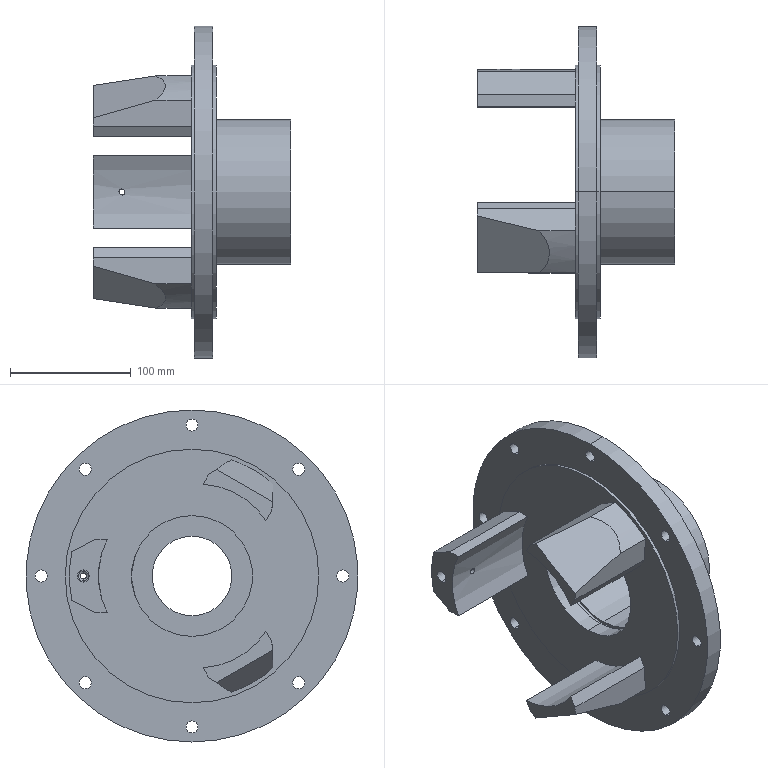Part | STEP file | Input 16 | 1 solid | 86 faces | box 164 x 275 x 275 mm | volume 1448032 mm3 | cylinder 54 | plane 28 | cone 4 | commonest cylinder face diameters 10 x20 5 x8 8.5 x4 100.2 x4 210 x4 133 x3